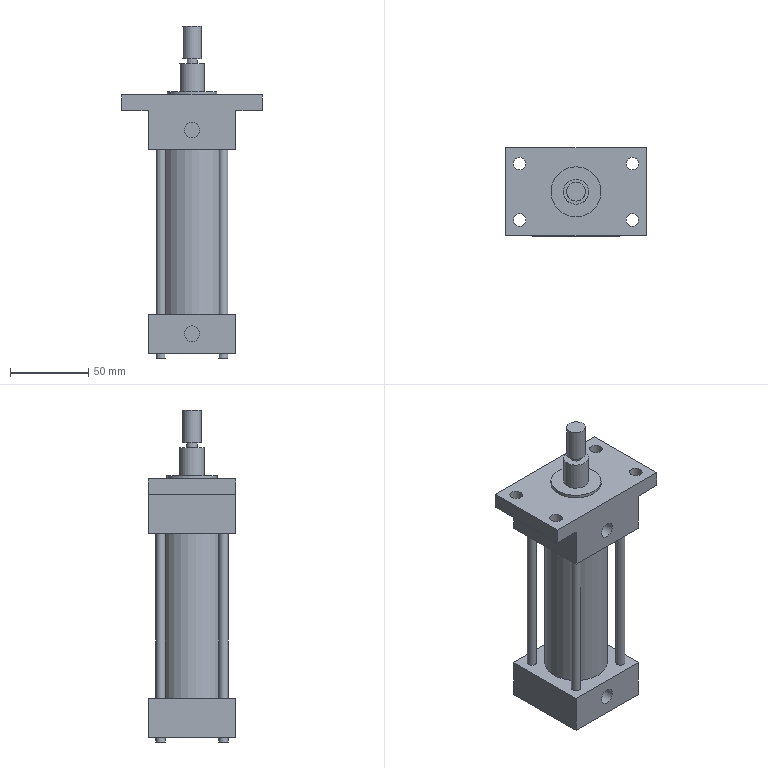Part | NX | features solid 2 | 1 solid | 48 faces | box 90 x 56 x 212 mm | volume 266006 mm3 | plane 28 | cylinder 20 | commonest cylinder face diameters 6 x8 8 x4 10 x2 7 x1 12 x1 16 x1
STEP:
#1=CARTESIAN_POINT('',(0.,-225.,-150.));
#2=VERTEX_POINT('',#1);
#3=CARTESIAN_POINT('',(0.,-245.,-150.));
#4=DIRECTION('',(0.,0.,1.));
#5=DIRECTION('',(0.,1.,0.));
#6=AXIS2_PLACEMENT_3D('',#3,#4,#5);
#7=CIRCLE('',#6,20.);
#8=EDGE_CURVE('',#2,#2,#7,.T.);
#9=ORIENTED_EDGE('',*,*,#8,.F.);
#10=EDGE_LOOP('',(#9));
#11=FACE_BOUND('',#10,.T.);
#12=CARTESIAN_POINT('',(0.,-225.,-255.));
#13=VERTEX_POINT('',#12);
#14=CARTESIAN_POINT('',(0.,-245.,-255.));
#15=DIRECTION('',(0.,0.,1.));
#16=DIRECTION('',(0.,1.,0.));
#17=AXIS2_PLACEMENT_3D('',#14,#15,#16);
#18=CIRCLE('',#17,20.);
#19=EDGE_CURVE('',#13,#13,#18,.F.);
#20=ORIENTED_EDGE('',*,*,#19,.F.);
#21=EDGE_LOOP('',(#20));
#22=FACE_BOUND('',#21,.T.);
#23=CARTESIAN_POINT('',(0.,-245.,-280.));
#24=DIRECTION('',(0.,0.,1.));
#25=DIRECTION('',(0.,-1.,0.));
#26=AXIS2_PLACEMENT_3D('',#23,#24,#25);
#27=CYLINDRICAL_SURFACE('',#26,20.);
#28=ADVANCED_FACE('',(#11,#22),#27,.T.);
#29=CARTESIAN_POINT('',(0.,-253.,-95.));
#30=VERTEX_POINT('',#29);
#31=CARTESIAN_POINT('',(0.,-245.,-95.));
#32=DIRECTION('',(0.,0.,-1.));
#33=DIRECTION('',(0.,-1.,0.));
#34=AXIS2_PLACEMENT_3D('',#31,#32,#33);
#35=CIRCLE('',#34,8.);
#36=EDGE_CURVE('',#30,#30,#35,.T.);
#37=ORIENTED_EDGE('',*,*,#36,.F.);
#38=EDGE_LOOP('',(#37));
#39=FACE_BOUND('',#38,.T.);
#40=CARTESIAN_POINT('',(0.,-248.5,-95.));
#41=VERTEX_POINT('',#40);
#42=CARTESIAN_POINT('',(0.,-245.,-95.));
#43=DIRECTION('',(0.,0.,-1.));
#44=DIRECTION('',(0.,-1.,0.));
#45=AXIS2_PLACEMENT_3D('',#42,#43,#44);
#46=CIRCLE('',#45,3.5);
#47=EDGE_CURVE('',#41,#41,#46,.T.);
#48=ORIENTED_EDGE('',*,*,#47,.T.);
#49=EDGE_LOOP('',(#48));
#50=FACE_BOUND('',#49,.T.);
#51=CARTESIAN_POINT('',(0.,-245.,-95.));
#52=DIRECTION('',(0.,0.,1.));
#53=DIRECTION('',(0.,-1.,0.));
#54=AXIS2_PLACEMENT_3D('',#51,#52,#53);
#55=PLANE('',#54);
#56=ADVANCED_FACE('',(#39,#50),#55,.T.);
#57=CARTESIAN_POINT('',(0.,-261.,-113.));
#58=VERTEX_POINT('',#57);
#59=CARTESIAN_POINT('',(0.,-245.,-113.));
#60=DIRECTION('',(0.,0.,-1.));
#61=DIRECTION('',(0.,-1.,0.));
#62=AXIS2_PLACEMENT_3D('',#59,#60,#61);
#63=CIRCLE('',#62,16.);
#64=EDGE_CURVE('',#58,#58,#63,.T.);
#65=ORIENTED_EDGE('',*,*,#64,.F.);
#66=EDGE_LOOP('',(#65));
#67=FACE_BOUND('',#66,.T.);
#68=CARTESIAN_POINT('',(0.,-253.,-113.));
#69=VERTEX_POINT('',#68);
#70=CARTESIAN_POINT('',(0.,-245.,-113.));
#71=DIRECTION('',(0.,0.,-1.));
#72=DIRECTION('',(0.,-1.,0.));
#73=AXIS2_PLACEMENT_3D('',#70,#71,#72);
#74=CIRCLE('',#73,8.);
#75=EDGE_CURVE('',#69,#69,#74,.F.);
#76=ORIENTED_EDGE('',*,*,#75,.F.);
#77=EDGE_LOOP('',(#76));
#78=FACE_BOUND('',#77,.T.);
#79=CARTESIAN_POINT('',(0.,-245.,-113.));
#80=DIRECTION('',(0.,0.,1.));
#81=DIRECTION('',(0.,-1.,0.));
#82=AXIS2_PLACEMENT_3D('',#79,#80,#81);
#83=PLANE('',#82);
#84=ADVANCED_FACE('',(#67,#78),#83,.T.);
#85=CARTESIAN_POINT('',(-36.,-231.,-115.));
#86=VERTEX_POINT('',#85);
#87=CARTESIAN_POINT('',(-36.,-227.,-115.));
#88=DIRECTION('',(0.,0.,-1.));
#89=DIRECTION('',(0.,-1.,0.));
#90=AXIS2_PLACEMENT_3D('',#87,#88,#89);
#91=CIRCLE('',#90,4.);
#92=EDGE_CURVE('',#86,#86,#91,.T.);
#93=ORIENTED_EDGE('',*,*,#92,.T.);
#94=EDGE_LOOP('',(#93));
#95=FACE_BOUND('',#94,.T.);
#96=CARTESIAN_POINT('',(36.,-267.,-115.));
#97=VERTEX_POINT('',#96);
#98=CARTESIAN_POINT('',(36.,-263.,-115.));
#99=DIRECTION('',(0.,0.,-1.));
#100=DIRECTION('',(0.,-1.,0.));
#101=AXIS2_PLACEMENT_3D('',#98,#99,#100);
#102=CIRCLE('',#101,4.);
#103=EDGE_CURVE('',#97,#97,#102,.T.);
#104=ORIENTED_EDGE('',*,*,#103,.T.);
#105=EDGE_LOOP('',(#104));
#106=FACE_BOUND('',#105,.T.);
#107=CARTESIAN_POINT('',(-45.,-217.,-115.));
#108=VERTEX_POINT('',#107);
#109=CARTESIAN_POINT('',(-45.,-273.,-115.));
#110=VERTEX_POINT('',#109);
#111=CARTESIAN_POINT('',(-45.,-217.,-115.));
#112=DIRECTION('',(0.,-1.,0.));
#113=VECTOR('',#112,1000.);
#114=LINE('',#111,#113);
#115=EDGE_CURVE('',#108,#110,#114,.T.);
#116=ORIENTED_EDGE('',*,*,#115,.T.);
#117=CARTESIAN_POINT('',(45.,-273.,-115.));
#118=VERTEX_POINT('',#117);
#119=CARTESIAN_POINT('',(45.,-273.,-115.));
#120=DIRECTION('',(-1.,0.,0.));
#121=VECTOR('',#120,1000.);
#122=LINE('',#119,#121);
#123=EDGE_CURVE('',#118,#110,#122,.T.);
#124=ORIENTED_EDGE('',*,*,#123,.F.);
#125=CARTESIAN_POINT('',(45.,-217.,-115.));
#126=VERTEX_POINT('',#125);
#127=CARTESIAN_POINT('',(45.,-217.,-115.));
#128=DIRECTION('',(0.,-1.,0.));
#129=VECTOR('',#128,1000.);
#130=LINE('',#127,#129);
#131=EDGE_CURVE('',#126,#118,#130,.T.);
#132=ORIENTED_EDGE('',*,*,#131,.F.);
#133=CARTESIAN_POINT('',(-28.,-217.,-115.));
#134=DIRECTION('',(-1.,0.,0.));
#135=VECTOR('',#134,1000.);
#136=LINE('',#133,#135);
#137=EDGE_CURVE('',#126,#108,#136,.T.);
#138=ORIENTED_EDGE('',*,*,#137,.T.);
#139=EDGE_LOOP('',(#116,#124,#132,#138));
#140=FACE_BOUND('',#139,.T.);
#141=CARTESIAN_POINT('',(36.,-231.,-115.));
#142=VERTEX_POINT('',#141);
#143=CARTESIAN_POINT('',(36.,-227.,-115.));
#144=DIRECTION('',(0.,0.,-1.));
#145=DIRECTION('',(0.,-1.,0.));
#146=AXIS2_PLACEMENT_3D('',#143,#144,#145);
#147=CIRCLE('',#146,4.);
#148=EDGE_CURVE('',#142,#142,#147,.T.);
#149=ORIENTED_EDGE('',*,*,#148,.T.);
#150=EDGE_LOOP('',(#149));
#151=FACE_BOUND('',#150,.T.);
#152=CARTESIAN_POINT('',(-36.,-267.,-115.));
#153=VERTEX_POINT('',#152);
#154=CARTESIAN_POINT('',(-36.,-263.,-115.));
#155=DIRECTION('',(0.,0.,-1.));
#156=DIRECTION('',(0.,-1.,0.));
#157=AXIS2_PLACEMENT_3D('',#154,#155,#156);
#158=CIRCLE('',#157,4.);
#159=EDGE_CURVE('',#153,#153,#158,.T.);
#160=ORIENTED_EDGE('',*,*,#159,.T.);
#161=EDGE_LOOP('',(#160));
#162=FACE_BOUND('',#161,.T.);
#163=CARTESIAN_POINT('',(0.,-229.,-115.));
#164=VERTEX_POINT('',#163);
#165=CARTESIAN_POINT('',(0.,-245.,-115.));
#166=DIRECTION('',(0.,0.,1.));
#167=DIRECTION('',(0.,1.,0.));
#168=AXIS2_PLACEMENT_3D('',#165,#166,#167);
#169=CIRCLE('',#168,16.);
#170=EDGE_CURVE('',#164,#164,#169,.F.);
#171=ORIENTED_EDGE('',*,*,#170,.T.);
#172=EDGE_LOOP('',(#171));
#173=FACE_BOUND('',#172,.T.);
#174=CARTESIAN_POINT('',(-45.,-273.,-115.));
#175=DIRECTION('',(0.,0.,-1.));
#176=DIRECTION('',(0.,1.,0.));
#177=AXIS2_PLACEMENT_3D('',#174,#175,#176);
#178=PLANE('',#177);
#179=ADVANCED_FACE('',(#95,#106,#140,#151,#162,#173),#178,.F.);
#180=CARTESIAN_POINT('',(28.,-273.,-125.));
#181=VERTEX_POINT('',#180);
#182=CARTESIAN_POINT('',(28.,-217.,-125.));
#183=VERTEX_POINT('',#182);
#184=CARTESIAN_POINT('',(28.,-273.,-125.));
#185=DIRECTION('',(0.,1.,0.));
#186=VECTOR('',#185,1000.);
#187=LINE('',#184,#186);
#188=EDGE_CURVE('',#181,#183,#187,.T.);
#189=ORIENTED_EDGE('',*,*,#188,.T.);
#190=CARTESIAN_POINT('',(45.,-217.,-125.));
#191=VERTEX_POINT('',#190);
#192=CARTESIAN_POINT('',(-28.,-217.,-125.));
#193=DIRECTION('',(-1.,0.,0.));
#194=VECTOR('',#193,1000.);
#195=LINE('',#192,#194);
#196=EDGE_CURVE('',#191,#183,#195,.T.);
#197=ORIENTED_EDGE('',*,*,#196,.F.);
#198=CARTESIAN_POINT('',(45.,-273.,-125.));
#199=VERTEX_POINT('',#198);
#200=CARTESIAN_POINT('',(45.,-217.,-125.));
#201=DIRECTION('',(0.,-1.,0.));
#202=VECTOR('',#201,1000.);
#203=LINE('',#200,#202);
#204=EDGE_CURVE('',#191,#199,#203,.T.);
#205=ORIENTED_EDGE('',*,*,#204,.T.);
#206=CARTESIAN_POINT('',(45.,-273.,-125.));
#207=DIRECTION('',(-1.,0.,0.));
#208=VECTOR('',#207,1000.);
#209=LINE('',#206,#208);
#210=EDGE_CURVE('',#199,#181,#209,.T.);
#211=ORIENTED_EDGE('',*,*,#210,.T.);
#212=EDGE_LOOP('',(#189,#197,#205,#211));
#213=FACE_BOUND('',#212,.T.);
#214=CARTESIAN_POINT('',(36.,-267.,-125.));
#215=VERTEX_POINT('',#214);
#216=CARTESIAN_POINT('',(36.,-263.,-125.));
#217=DIRECTION('',(0.,0.,-1.));
#218=DIRECTION('',(0.,-1.,0.));
#219=AXIS2_PLACEMENT_3D('',#216,#217,#218);
#220=CIRCLE('',#219,4.);
#221=EDGE_CURVE('',#215,#215,#220,.T.);
#222=ORIENTED_EDGE('',*,*,#221,.F.);
#223=EDGE_LOOP('',(#222));
#224=FACE_BOUND('',#223,.T.);
#225=CARTESIAN_POINT('',(36.,-231.,-125.));
#226=VERTEX_POINT('',#225);
#227=CARTESIAN_POINT('',(36.,-227.,-125.));
#228=DIRECTION('',(0.,0.,-1.));
#229=DIRECTION('',(0.,-1.,0.));
#230=AXIS2_PLACEMENT_3D('',#227,#228,#229);
#231=CIRCLE('',#230,4.);
#232=EDGE_CURVE('',#226,#226,#231,.T.);
#233=ORIENTED_EDGE('',*,*,#232,.F.);
#234=EDGE_LOOP('',(#233));
#235=FACE_BOUND('',#234,.T.);
#236=CARTESIAN_POINT('',(-45.,-273.,-125.));
#237=DIRECTION('',(0.,0.,-1.));
#238=DIRECTION('',(0.,1.,0.));
#239=AXIS2_PLACEMENT_3D('',#236,#237,#238);
#240=PLANE('',#239);
#241=ADVANCED_FACE('',(#213,#224,#235),#240,.T.);
#242=ORIENTED_EDGE('',*,*,#115,.F.);
#243=CARTESIAN_POINT('',(-45.,-217.,-125.));
#244=VERTEX_POINT('',#243);
#245=CARTESIAN_POINT('',(-45.,-217.,-125.));
#246=DIRECTION('',(0.,0.,1.));
#247=VECTOR('',#246,1000.);
#248=LINE('',#245,#247);
#249=EDGE_CURVE('',#244,#108,#248,.T.);
#250=ORIENTED_EDGE('',*,*,#249,.F.);
#251=CARTESIAN_POINT('',(-45.,-273.,-125.));
#252=VERTEX_POINT('',#251);
#253=CARTESIAN_POINT('',(-45.,-217.,-125.));
#254=DIRECTION('',(0.,-1.,0.));
#255=VECTOR('',#254,1000.);
#256=LINE('',#253,#255);
#257=EDGE_CURVE('',#244,#252,#256,.T.);
#258=ORIENTED_EDGE('',*,*,#257,.T.);
#259=CARTESIAN_POINT('',(-45.,-273.,-125.));
#260=DIRECTION('',(0.,0.,1.));
#261=VECTOR('',#260,1000.);
#262=LINE('',#259,#261);
#263=EDGE_CURVE('',#252,#110,#262,.T.);
#264=ORIENTED_EDGE('',*,*,#263,.T.);
#265=EDGE_LOOP('',(#242,#250,#258,#264));
#266=FACE_BOUND('',#265,.T.);
#267=CARTESIAN_POINT('',(-45.,-217.,-125.));
#268=DIRECTION('',(1.,0.,0.));
#269=DIRECTION('',(0.,0.,-1.));
#270=AXIS2_PLACEMENT_3D('',#267,#268,#269);
#271=PLANE('',#270);
#272=ADVANCED_FACE('',(#266),#271,.F.);
#273=CARTESIAN_POINT('',(5.,-273.,-137.5));
#274=VERTEX_POINT('',#273);
#275=CARTESIAN_POINT('',(0.,-273.,-137.5));
#276=DIRECTION('',(0.,-1.,0.));
#277=DIRECTION('',(1.,0.,0.));
#278=AXIS2_PLACEMENT_3D('',#275,#276,#277);
#279=CIRCLE('',#278,5.);
#280=EDGE_CURVE('',#274,#274,#279,.T.);
#281=ORIENTED_EDGE('',*,*,#280,.F.);
#282=EDGE_LOOP('',(#281));
#283=FACE_BOUND('',#282,.T.);
#284=ORIENTED_EDGE('',*,*,#123,.T.);
#285=ORIENTED_EDGE('',*,*,#263,.F.);
#286=CARTESIAN_POINT('',(-28.,-273.,-125.));
#287=VERTEX_POINT('',#286);
#288=CARTESIAN_POINT('',(45.,-273.,-125.));
#289=DIRECTION('',(-1.,0.,0.));
#290=VECTOR('',#289,1000.);
#291=LINE('',#288,#290);
#292=EDGE_CURVE('',#287,#252,#291,.T.);
#293=ORIENTED_EDGE('',*,*,#292,.F.);
#294=CARTESIAN_POINT('',(-28.,-273.,-150.));
#295=VERTEX_POINT('',#294);
#296=CARTESIAN_POINT('',(-28.,-273.,-150.));
#297=DIRECTION('',(0.,0.,1.));
#298=VECTOR('',#297,1000.);
#299=LINE('',#296,#298);
#300=EDGE_CURVE('',#295,#287,#299,.T.);
#301=ORIENTED_EDGE('',*,*,#300,.F.);
#302=CARTESIAN_POINT('',(28.,-273.,-150.));
#303=VERTEX_POINT('',#302);
#304=CARTESIAN_POINT('',(-28.,-273.,-150.));
#305=DIRECTION('',(1.,0.,0.));
#306=VECTOR('',#305,1000.);
#307=LINE('',#304,#306);
#308=EDGE_CURVE('',#295,#303,#307,.T.);
#309=ORIENTED_EDGE('',*,*,#308,.T.);
#310=CARTESIAN_POINT('',(28.,-273.,-150.));
#311=DIRECTION('',(0.,0.,1.));
#312=VECTOR('',#311,1000.);
#313=LINE('',#310,#312);
#314=EDGE_CURVE('',#303,#181,#313,.T.);
#315=ORIENTED_EDGE('',*,*,#314,.T.);
#316=ORIENTED_EDGE('',*,*,#210,.F.);
#317=CARTESIAN_POINT('',(45.,-273.,-125.));
#318=DIRECTION('',(0.,0.,1.));
#319=VECTOR('',#318,1000.);
#320=LINE('',#317,#319);
#321=EDGE_CURVE('',#199,#118,#320,.T.);
#322=ORIENTED_EDGE('',*,*,#321,.T.);
#323=EDGE_LOOP('',(#284,#285,#293,#301,#309,#315,#316,#322));
#324=FACE_BOUND('',#323,.T.);
#325=CARTESIAN_POINT('',(45.,-273.,-125.));
#326=DIRECTION('',(0.,-1.,0.));
#327=DIRECTION('',(-1.,0.,0.));
#328=AXIS2_PLACEMENT_3D('',#325,#326,#327);
#329=PLANE('',#328);
#330=ADVANCED_FACE('',(#283,#324),#329,.T.);
#331=ORIENTED_EDGE('',*,*,#131,.T.);
#332=ORIENTED_EDGE('',*,*,#321,.F.);
#333=ORIENTED_EDGE('',*,*,#204,.F.);
#334=CARTESIAN_POINT('',(45.,-217.,-125.));
#335=DIRECTION('',(0.,0.,1.));
#336=VECTOR('',#335,1000.);
#337=LINE('',#334,#336);
#338=EDGE_CURVE('',#191,#126,#337,.T.);
#339=ORIENTED_EDGE('',*,*,#338,.T.);
#340=EDGE_LOOP('',(#331,#332,#333,#339));
#341=FACE_BOUND('',#340,.T.);
#342=CARTESIAN_POINT('',(45.,-217.,-125.));
#343=DIRECTION('',(1.,0.,0.));
#344=DIRECTION('',(0.,0.,-1.));
#345=AXIS2_PLACEMENT_3D('',#342,#343,#344);
#346=PLANE('',#345);
#347=ADVANCED_FACE('',(#341),#346,.T.);
#348=ORIENTED_EDGE('',*,*,#221,.T.);
#349=EDGE_LOOP('',(#348));
#350=FACE_BOUND('',#349,.T.);
#351=ORIENTED_EDGE('',*,*,#103,.F.);
#352=EDGE_LOOP('',(#351));
#353=FACE_BOUND('',#352,.T.);
#354=CARTESIAN_POINT('',(36.,-263.,-125.));
#355=DIRECTION('',(0.,0.,1.));
#356=DIRECTION('',(0.,-1.,0.));
#357=AXIS2_PLACEMENT_3D('',#354,#355,#356);
#358=CYLINDRICAL_SURFACE('',#357,4.);
#359=ADVANCED_FACE('',(#350,#353),#358,.F.);
#360=ORIENTED_EDGE('',*,*,#137,.F.);
#361=ORIENTED_EDGE('',*,*,#338,.F.);
#362=ORIENTED_EDGE('',*,*,#196,.T.);
#363=CARTESIAN_POINT('',(28.,-217.,-150.));
#364=VERTEX_POINT('',#363);
#365=CARTESIAN_POINT('',(28.,-217.,-150.));
#366=DIRECTION('',(0.,0.,1.));
#367=VECTOR('',#366,1000.);
#368=LINE('',#365,#367);
#369=EDGE_CURVE('',#364,#183,#368,.T.);
#370=ORIENTED_EDGE('',*,*,#369,.F.);
#371=CARTESIAN_POINT('',(-28.,-217.,-150.));
#372=VERTEX_POINT('',#371);
#373=CARTESIAN_POINT('',(28.,-217.,-150.));
#374=DIRECTION('',(-1.,0.,0.));
#375=VECTOR('',#374,1000.);
#376=LINE('',#373,#375);
#377=EDGE_CURVE('',#364,#372,#376,.T.);
#378=ORIENTED_EDGE('',*,*,#377,.T.);
#379=CARTESIAN_POINT('',(-28.,-217.,-125.));
#380=VERTEX_POINT('',#379);
#381=CARTESIAN_POINT('',(-28.,-217.,-150.));
#382=DIRECTION('',(0.,0.,1.));
#383=VECTOR('',#382,1000.);
#384=LINE('',#381,#383);
#385=EDGE_CURVE('',#372,#380,#384,.T.);
#386=ORIENTED_EDGE('',*,*,#385,.T.);
#387=CARTESIAN_POINT('',(-28.,-217.,-125.));
#388=DIRECTION('',(-1.,0.,0.));
#389=VECTOR('',#388,1000.);
#390=LINE('',#387,#389);
#391=EDGE_CURVE('',#380,#244,#390,.T.);
#392=ORIENTED_EDGE('',*,*,#391,.T.);
#393=ORIENTED_EDGE('',*,*,#249,.T.);
#394=EDGE_LOOP('',(#360,#361,#362,#370,#378,#386,#392,#393));
#395=FACE_BOUND('',#394,.T.);
#396=CARTESIAN_POINT('',(-28.,-217.,-125.));
#397=DIRECTION('',(0.,-1.,0.));
#398=DIRECTION('',(0.,0.,-1.));
#399=AXIS2_PLACEMENT_3D('',#396,#397,#398);
#400=PLANE('',#399);
#401=ADVANCED_FACE('',(#395),#400,.F.);
#402=ORIENTED_EDGE('',*,*,#232,.T.);
#403=EDGE_LOOP('',(#402));
#404=FACE_BOUND('',#403,.T.);
#405=ORIENTED_EDGE('',*,*,#148,.F.);
#406=EDGE_LOOP('',(#405));
#407=FACE_BOUND('',#406,.T.);
#408=CARTESIAN_POINT('',(36.,-227.,-125.));
#409=DIRECTION('',(0.,0.,1.));
#410=DIRECTION('',(0.,-1.,0.));
#411=AXIS2_PLACEMENT_3D('',#408,#409,#410);
#412=CYLINDRICAL_SURFACE('',#411,4.);
#413=ADVANCED_FACE('',(#404,#407),#412,.F.);
#414=CARTESIAN_POINT('',(-36.,-267.,-125.));
#415=VERTEX_POINT('',#414);
#416=CARTESIAN_POINT('',(-36.,-263.,-125.));
#417=DIRECTION('',(0.,0.,-1.));
#418=DIRECTION('',(0.,-1.,0.));
#419=AXIS2_PLACEMENT_3D('',#416,#417,#418);
#420=CIRCLE('',#419,4.);
#421=EDGE_CURVE('',#415,#415,#420,.T.);
#422=ORIENTED_EDGE('',*,*,#421,.T.);
#423=EDGE_LOOP('',(#422));
#424=FACE_BOUND('',#423,.T.);
#425=ORIENTED_EDGE('',*,*,#159,.F.);
#426=EDGE_LOOP('',(#425));
#427=FACE_BOUND('',#426,.T.);
#428=CARTESIAN_POINT('',(-36.,-263.,-125.));
#429=DIRECTION('',(0.,0.,1.));
#430=DIRECTION('',(0.,-1.,0.));
#431=AXIS2_PLACEMENT_3D('',#428,#429,#430);
#432=CYLINDRICAL_SURFACE('',#431,4.);
#433=ADVANCED_FACE('',(#424,#427),#432,.F.);
#434=CARTESIAN_POINT('',(-36.,-231.,-125.));
#435=VERTEX_POINT('',#434);
#436=CARTESIAN_POINT('',(-36.,-227.,-125.));
#437=DIRECTION('',(0.,0.,-1.));
#438=DIRECTION('',(0.,-1.,0.));
#439=AXIS2_PLACEMENT_3D('',#436,#437,#438);
#440=CIRCLE('',#439,4.);
#441=EDGE_CURVE('',#435,#435,#440,.T.);
#442=ORIENTED_EDGE('',*,*,#441,.T.);
#443=EDGE_LOOP('',(#442));
#444=FACE_BOUND('',#443,.T.);
#445=ORIENTED_EDGE('',*,*,#92,.F.);
#446=EDGE_LOOP('',(#445));
#447=FACE_BOUND('',#446,.T.);
#448=CARTESIAN_POINT('',(-36.,-227.,-125.));
#449=DIRECTION('',(0.,0.,1.));
#450=DIRECTION('',(0.,-1.,0.));
#451=AXIS2_PLACEMENT_3D('',#448,#449,#450);
#452=CYLINDRICAL_SURFACE('',#451,4.);
#453=ADVANCED_FACE('',(#444,#447),#452,.F.);
#454=CARTESIAN_POINT('',(-28.,-217.,-125.));
#455=DIRECTION('',(0.,-1.,0.));
#456=VECTOR('',#455,1000.);
#457=LINE('',#454,#456);
#458=EDGE_CURVE('',#380,#287,#457,.T.);
#459=ORIENTED_EDGE('',*,*,#458,.T.);
#460=ORIENTED_EDGE('',*,*,#292,.T.);
#461=ORIENTED_EDGE('',*,*,#257,.F.);
#462=ORIENTED_EDGE('',*,*,#391,.F.);
#463=EDGE_LOOP('',(#459,#460,#461,#462));
#464=FACE_BOUND('',#463,.T.);
#465=ORIENTED_EDGE('',*,*,#421,.F.);
#466=EDGE_LOOP('',(#465));
#467=FACE_BOUND('',#466,.T.);
#468=ORIENTED_EDGE('',*,*,#441,.F.);
#469=EDGE_LOOP('',(#468));
#470=FACE_BOUND('',#469,.T.);
#471=CARTESIAN_POINT('',(-45.,-273.,-125.));
#472=DIRECTION('',(0.,0.,-1.));
#473=DIRECTION('',(0.,1.,0.));
#474=AXIS2_PLACEMENT_3D('',#471,#472,#473);
#475=PLANE('',#474);
#476=ADVANCED_FACE('',(#464,#467,#470),#475,.T.);
#477=ORIENTED_EDGE('',*,*,#458,.F.);
#478=ORIENTED_EDGE('',*,*,#385,.F.);
#479=CARTESIAN_POINT('',(-28.,-217.,-150.));
#480=DIRECTION('',(0.,-1.,0.));
#481=VECTOR('',#480,1000.);
#482=LINE('',#479,#481);
#483=EDGE_CURVE('',#372,#295,#482,.T.);
#484=ORIENTED_EDGE('',*,*,#483,.T.);
#485=ORIENTED_EDGE('',*,*,#300,.T.);
#486=EDGE_LOOP('',(#477,#478,#484,#485));
#487=FACE_BOUND('',#486,.T.);
#488=CARTESIAN_POINT('',(-28.,-217.,-150.));
#489=DIRECTION('',(1.,0.,0.));
#490=DIRECTION('',(0.,0.,-1.));
#491=AXIS2_PLACEMENT_3D('',#488,#489,#490);
#492=PLANE('',#491);
#493=ADVANCED_FACE('',(#487),#492,.F.);
#494=ORIENTED_EDGE('',*,*,#188,.F.);
#495=ORIENTED_EDGE('',*,*,#314,.F.);
#496=CARTESIAN_POINT('',(28.,-273.,-150.));
#497=DIRECTION('',(0.,1.,0.));
#498=VECTOR('',#497,1000.);
#499=LINE('',#496,#498);
#500=EDGE_CURVE('',#303,#364,#499,.T.);
#501=ORIENTED_EDGE('',*,*,#500,.T.);
#502=ORIENTED_EDGE('',*,*,#369,.T.);
#503=EDGE_LOOP('',(#494,#495,#501,#502));
#504=FACE_BOUND('',#503,.T.);
#505=CARTESIAN_POINT('',(28.,-273.,-150.));
#506=DIRECTION('',(-1.,0.,0.));
#507=DIRECTION('',(0.,0.,1.));
#508=AXIS2_PLACEMENT_3D('',#505,#506,#507);
#509=PLANE('',#508);
#510=ADVANCED_FACE('',(#504),#509,.F.);
#511=CARTESIAN_POINT('',(-20.,-262.,-150.));
#512=VERTEX_POINT('',#511);
#513=CARTESIAN_POINT('',(-20.,-265.,-150.));
#514=DIRECTION('',(0.,0.,1.));
#515=DIRECTION('',(0.,1.,0.));
#516=AXIS2_PLACEMENT_3D('',#513,#514,#515);
#517=CIRCLE('',#516,3.);
#518=EDGE_CURVE('',#512,#512,#517,.T.);
#519=ORIENTED_EDGE('',*,*,#518,.T.);
#520=EDGE_LOOP('',(#519));
#521=FACE_BOUND('',#520,.T.);
#522=CARTESIAN_POINT('',(-20.,-222.,-150.));
#523=VERTEX_POINT('',#522);
#524=CARTESIAN_POINT('',(-20.,-225.,-150.));
#525=DIRECTION('',(0.,0.,1.));
#526=DIRECTION('',(0.,1.,0.));
#527=AXIS2_PLACEMENT_3D('',#524,#525,#526);
#528=CIRCLE('',#527,3.);
#529=EDGE_CURVE('',#523,#523,#528,.T.);
#530=ORIENTED_EDGE('',*,*,#529,.T.);
#531=EDGE_LOOP('',(#530));
#532=FACE_BOUND('',#531,.T.);
#533=CARTESIAN_POINT('',(20.,-222.,-150.));
#534=VERTEX_POINT('',#533);
#535=CARTESIAN_POINT('',(20.,-225.,-150.));
#536=DIRECTION('',(0.,0.,1.));
#537=DIRECTION('',(0.,1.,0.));
#538=AXIS2_PLACEMENT_3D('',#535,#536,#537);
#539=CIRCLE('',#538,3.);
#540=EDGE_CURVE('',#534,#534,#539,.T.);
#541=ORIENTED_EDGE('',*,*,#540,.T.);
#542=EDGE_LOOP('',(#541));
#543=FACE_BOUND('',#542,.T.);
#544=CARTESIAN_POINT('',(20.,-262.,-150.));
#545=VERTEX_POINT('',#544);
#546=CARTESIAN_POINT('',(20.,-265.,-150.));
#547=DIRECTION('',(0.,0.,1.));
#548=DIRECTION('',(0.,1.,0.));
#549=AXIS2_PLACEMENT_3D('',#546,#547,#548);
#550=CIRCLE('',#549,3.);
#551=EDGE_CURVE('',#545,#545,#550,.T.);
#552=ORIENTED_EDGE('',*,*,#551,.T.);
#553=EDGE_LOOP('',(#552));
#554=FACE_BOUND('',#553,.T.);
#555=ORIENTED_EDGE('',*,*,#8,.T.);
#556=EDGE_LOOP('',(#555));
#557=FACE_BOUND('',#556,.T.);
#558=ORIENTED_EDGE('',*,*,#377,.F.);
#559=ORIENTED_EDGE('',*,*,#500,.F.);
#560=ORIENTED_EDGE('',*,*,#308,.F.);
#561=ORIENTED_EDGE('',*,*,#483,.F.);
#562=EDGE_LOOP('',(#558,#559,#560,#561));
#563=FACE_BOUND('',#562,.T.);
#564=CARTESIAN_POINT('',(-28.,-217.,-150.));
#565=DIRECTION('',(0.,0.,-1.));
#566=DIRECTION('',(0.,1.,0.));
#567=AXIS2_PLACEMENT_3D('',#564,#565,#566);
#568=PLANE('',#567);
#569=ADVANCED_FACE('',(#521,#532,#543,#554,#557,#563),#568,.T.);
#570=ORIENTED_EDGE('',*,*,#64,.T.);
#571=EDGE_LOOP('',(#570));
#572=FACE_BOUND('',#571,.T.);
#573=ORIENTED_EDGE('',*,*,#170,.F.);
#574=EDGE_LOOP('',(#573));
#575=FACE_BOUND('',#574,.T.);
#576=CARTESIAN_POINT('',(0.,-245.,-113.));
#577=DIRECTION('',(0.,0.,-1.));
#578=DIRECTION('',(0.,1.,0.));
#579=AXIS2_PLACEMENT_3D('',#576,#577,#578);
#580=CYLINDRICAL_SURFACE('',#579,16.);
#581=ADVANCED_FACE('',(#572,#575),#580,.T.);
#582=ORIENTED_EDGE('',*,*,#75,.T.);
#583=EDGE_LOOP('',(#582));
#584=FACE_BOUND('',#583,.T.);
#585=ORIENTED_EDGE('',*,*,#36,.T.);
#586=EDGE_LOOP('',(#585));
#587=FACE_BOUND('',#586,.T.);
#588=CARTESIAN_POINT('',(0.,-245.,-95.));
#589=DIRECTION('',(0.,0.,-1.));
#590=DIRECTION('',(0.,1.,0.));
#591=AXIS2_PLACEMENT_3D('',#588,#589,#590);
#592=CYLINDRICAL_SURFACE('',#591,8.);
#593=ADVANCED_FACE('',(#584,#587),#592,.T.);
#594=CARTESIAN_POINT('',(28.,-217.,-255.));
#595=VERTEX_POINT('',#594);
#596=CARTESIAN_POINT('',(-28.,-217.,-255.));
#597=VERTEX_POINT('',#596);
#598=CARTESIAN_POINT('',(28.,-217.,-255.));
#599=DIRECTION('',(-1.,0.,0.));
#600=VECTOR('',#599,1000.);
#601=LINE('',#598,#600);
#602=EDGE_CURVE('',#595,#597,#601,.T.);
#603=ORIENTED_EDGE('',*,*,#602,.F.);
#604=CARTESIAN_POINT('',(28.,-217.,-280.));
#605=VERTEX_POINT('',#604);
#606=CARTESIAN_POINT('',(28.,-217.,-280.));
#607=DIRECTION('',(0.,0.,1.));
#608=VECTOR('',#607,1000.);
#609=LINE('',#606,#608);
#610=EDGE_CURVE('',#605,#595,#609,.T.);
#611=ORIENTED_EDGE('',*,*,#610,.F.);
#612=CARTESIAN_POINT('',(-28.,-217.,-280.));
#613=VERTEX_POINT('',#612);
#614=CARTESIAN_POINT('',(28.,-217.,-280.));
#615=DIRECTION('',(-1.,0.,0.));
#616=VECTOR('',#615,1000.);
#617=LINE('',#614,#616);
#618=EDGE_CURVE('',#605,#613,#617,.T.);
#619=ORIENTED_EDGE('',*,*,#618,.T.);
#620=CARTESIAN_POINT('',(-28.,-217.,-280.));
#621=DIRECTION('',(0.,0.,1.));
#622=VECTOR('',#621,1000.);
#623=LINE('',#620,#622);
#624=EDGE_CURVE('',#613,#597,#623,.T.);
#625=ORIENTED_EDGE('',*,*,#624,.T.);
#626=EDGE_LOOP('',(#603,#611,#619,#625));
#627=FACE_BOUND('',#626,.T.);
#628=CARTESIAN_POINT('',(28.,-217.,-280.));
#629=DIRECTION('',(0.,-1.,0.));
#630=DIRECTION('',(0.,0.,-1.));
#631=AXIS2_PLACEMENT_3D('',#628,#629,#630);
#632=PLANE('',#631);
#633=ADVANCED_FACE('',(#627),#632,.F.);
#634=CARTESIAN_POINT('',(-28.,-273.,-255.));
#635=VERTEX_POINT('',#634);
#636=CARTESIAN_POINT('',(-28.,-217.,-255.));
#637=DIRECTION('',(0.,-1.,0.));
#638=VECTOR('',#637,1000.);
#639=LINE('',#636,#638);
#640=EDGE_CURVE('',#597,#635,#639,.T.);
#641=ORIENTED_EDGE('',*,*,#640,.F.);
#642=ORIENTED_EDGE('',*,*,#624,.F.);
#643=CARTESIAN_POINT('',(-28.,-273.,-280.));
#644=VERTEX_POINT('',#643);
#645=CARTESIAN_POINT('',(-28.,-217.,-280.));
#646=DIRECTION('',(0.,-1.,0.));
#647=VECTOR('',#646,1000.);
#648=LINE('',#645,#647);
#649=EDGE_CURVE('',#613,#644,#648,.T.);
#650=ORIENTED_EDGE('',*,*,#649,.T.);
#651=CARTESIAN_POINT('',(-28.,-273.,-280.));
#652=DIRECTION('',(0.,0.,1.));
#653=VECTOR('',#652,1000.);
#654=LINE('',#651,#653);
#655=EDGE_CURVE('',#644,#635,#654,.T.);
#656=ORIENTED_EDGE('',*,*,#655,.T.);
#657=EDGE_LOOP('',(#641,#642,#650,#656));
#658=FACE_BOUND('',#657,.T.);
#659=CARTESIAN_POINT('',(-28.,-217.,-280.));
#660=DIRECTION('',(1.,0.,0.));
#661=DIRECTION('',(0.,0.,-1.));
#662=AXIS2_PLACEMENT_3D('',#659,#660,#661);
#663=PLANE('',#662);
#664=ADVANCED_FACE('',(#658),#663,.F.);
#665=CARTESIAN_POINT('',(5.,-273.,-267.5));
#666=VERTEX_POINT('',#665);
#667=CARTESIAN_POINT('',(0.,-273.,-267.5));
#668=DIRECTION('',(0.,-1.,0.));
#669=DIRECTION('',(1.,0.,0.));
#670=AXIS2_PLACEMENT_3D('',#667,#668,#669);
#671=CIRCLE('',#670,5.);
#672=EDGE_CURVE('',#666,#666,#671,.T.);
#673=ORIENTED_EDGE('',*,*,#672,.F.);
#674=EDGE_LOOP('',(#673));
#675=FACE_BOUND('',#674,.T.);
#676=CARTESIAN_POINT('',(28.,-273.,-255.));
#677=VERTEX_POINT('',#676);
#678=CARTESIAN_POINT('',(-28.,-273.,-255.));
#679=DIRECTION('',(1.,0.,0.));
#680=VECTOR('',#679,1000.);
#681=LINE('',#678,#680);
#682=EDGE_CURVE('',#635,#677,#681,.T.);
#683=ORIENTED_EDGE('',*,*,#682,.F.);
#684=ORIENTED_EDGE('',*,*,#655,.F.);
#685=CARTESIAN_POINT('',(28.,-273.,-280.));
#686=VERTEX_POINT('',#685);
#687=CARTESIAN_POINT('',(-28.,-273.,-280.));
#688=DIRECTION('',(1.,0.,0.));
#689=VECTOR('',#688,1000.);
#690=LINE('',#687,#689);
#691=EDGE_CURVE('',#644,#686,#690,.T.);
#692=ORIENTED_EDGE('',*,*,#691,.T.);
#693=CARTESIAN_POINT('',(28.,-273.,-280.));
#694=DIRECTION('',(0.,0.,1.));
#695=VECTOR('',#694,1000.);
#696=LINE('',#693,#695);
#697=EDGE_CURVE('',#686,#677,#696,.T.);
#698=ORIENTED_EDGE('',*,*,#697,.T.);
#699=EDGE_LOOP('',(#683,#684,#692,#698));
#700=FACE_BOUND('',#699,.T.);
#701=CARTESIAN_POINT('',(-28.,-273.,-280.));
#702=DIRECTION('',(0.,1.,0.));
#703=DIRECTION('',(1.,0.,0.));
#704=AXIS2_PLACEMENT_3D('',#701,#702,#703);
#705=PLANE('',#704);
#706=ADVANCED_FACE('',(#675,#700),#705,.F.);
#707=CARTESIAN_POINT('',(28.,-273.,-255.));
#708=DIRECTION('',(0.,1.,0.));
#709=VECTOR('',#708,1000.);
#710=LINE('',#707,#709);
#711=EDGE_CURVE('',#677,#595,#710,.T.);
#712=ORIENTED_EDGE('',*,*,#711,.F.);
#713=ORIENTED_EDGE('',*,*,#697,.F.);
#714=CARTESIAN_POINT('',(28.,-273.,-280.));
#715=DIRECTION('',(0.,1.,0.));
#716=VECTOR('',#715,1000.);
#717=LINE('',#714,#716);
#718=EDGE_CURVE('',#686,#605,#717,.T.);
#719=ORIENTED_EDGE('',*,*,#718,.T.);
#720=ORIENTED_EDGE('',*,*,#610,.T.);
#721=EDGE_LOOP('',(#712,#713,#719,#720));
#722=FACE_BOUND('',#721,.T.);
#723=CARTESIAN_POINT('',(28.,-273.,-280.));
#724=DIRECTION('',(-1.,0.,0.));
#725=DIRECTION('',(0.,0.,1.));
#726=AXIS2_PLACEMENT_3D('',#723,#724,#725);
#727=PLANE('',#726);
#728=ADVANCED_FACE('',(#722),#727,.F.);
#729=CARTESIAN_POINT('',(-20.,-262.,-255.));
#730=VERTEX_POINT('',#729);
#731=CARTESIAN_POINT('',(-20.,-265.,-255.));
#732=DIRECTION('',(0.,0.,1.));
#733=DIRECTION('',(0.,1.,0.));
#734=AXIS2_PLACEMENT_3D('',#731,#732,#733);
#735=CIRCLE('',#734,3.);
#736=EDGE_CURVE('',#730,#730,#735,.T.);
#737=ORIENTED_EDGE('',*,*,#736,.F.);
#738=EDGE_LOOP('',(#737));
#739=FACE_BOUND('',#738,.T.);
#740=CARTESIAN_POINT('',(-20.,-222.,-255.));
#741=VERTEX_POINT('',#740);
#742=CARTESIAN_POINT('',(-20.,-225.,-255.));
#743=DIRECTION('',(0.,0.,1.));
#744=DIRECTION('',(0.,1.,0.));
#745=AXIS2_PLACEMENT_3D('',#742,#743,#744);
#746=CIRCLE('',#745,3.);
#747=EDGE_CURVE('',#741,#741,#746,.T.);
#748=ORIENTED_EDGE('',*,*,#747,.F.);
#749=EDGE_LOOP('',(#748));
#750=FACE_BOUND('',#749,.T.);
#751=CARTESIAN_POINT('',(20.,-222.,-255.));
#752=VERTEX_POINT('',#751);
#753=CARTESIAN_POINT('',(20.,-225.,-255.));
#754=DIRECTION('',(0.,0.,1.));
#755=DIRECTION('',(0.,1.,0.));
#756=AXIS2_PLACEMENT_3D('',#753,#754,#755);
#757=CIRCLE('',#756,3.);
#758=EDGE_CURVE('',#752,#752,#757,.T.);
#759=ORIENTED_EDGE('',*,*,#758,.F.);
#760=EDGE_LOOP('',(#759));
#761=FACE_BOUND('',#760,.T.);
#762=CARTESIAN_POINT('',(20.,-262.,-255.));
#763=VERTEX_POINT('',#762);
#764=CARTESIAN_POINT('',(20.,-265.,-255.));
#765=DIRECTION('',(0.,0.,1.));
#766=DIRECTION('',(0.,1.,0.));
#767=AXIS2_PLACEMENT_3D('',#764,#765,#766);
#768=CIRCLE('',#767,3.);
#769=EDGE_CURVE('',#763,#763,#768,.T.);
#770=ORIENTED_EDGE('',*,*,#769,.F.);
#771=EDGE_LOOP('',(#770));
#772=FACE_BOUND('',#771,.T.);
#773=ORIENTED_EDGE('',*,*,#19,.T.);
#774=EDGE_LOOP('',(#773));
#775=FACE_BOUND('',#774,.T.);
#776=ORIENTED_EDGE('',*,*,#602,.T.);
#777=ORIENTED_EDGE('',*,*,#640,.T.);
#778=ORIENTED_EDGE('',*,*,#682,.T.);
#779=ORIENTED_EDGE('',*,*,#711,.T.);
#780=EDGE_LOOP('',(#776,#777,#778,#779));
#781=FACE_BOUND('',#780,.T.);
#782=CARTESIAN_POINT('',(-28.,-217.,-255.));
#783=DIRECTION('',(0.,0.,-1.));
#784=DIRECTION('',(0.,1.,0.));
#785=AXIS2_PLACEMENT_3D('',#782,#783,#784);
#786=PLANE('',#785);
#787=ADVANCED_FACE('',(#739,#750,#761,#772,#775,#781),#786,.F.);
#788=CARTESIAN_POINT('',(-20.,-268.,-280.));
#789=VERTEX_POINT('',#788);
#790=CARTESIAN_POINT('',(-20.,-265.,-280.));
#791=DIRECTION('',(0.,0.,-1.));
#792=DIRECTION('',(0.,-1.,0.));
#793=AXIS2_PLACEMENT_3D('',#790,#791,#792);
#794=CIRCLE('',#793,3.);
#795=EDGE_CURVE('',#789,#789,#794,.T.);
#796=ORIENTED_EDGE('',*,*,#795,.F.);
#797=EDGE_LOOP('',(#796));
#798=FACE_BOUND('',#797,.T.);
#799=CARTESIAN_POINT('',(-20.,-228.,-280.));
#800=VERTEX_POINT('',#799);
#801=CARTESIAN_POINT('',(-20.,-225.,-280.));
#802=DIRECTION('',(0.,0.,-1.));
#803=DIRECTION('',(0.,-1.,0.));
#804=AXIS2_PLACEMENT_3D('',#801,#802,#803);
#805=CIRCLE('',#804,3.);
#806=EDGE_CURVE('',#800,#800,#805,.T.);
#807=ORIENTED_EDGE('',*,*,#806,.F.);
#808=EDGE_LOOP('',(#807));
#809=FACE_BOUND('',#808,.T.);
#810=CARTESIAN_POINT('',(20.,-228.,-280.));
#811=VERTEX_POINT('',#810);
#812=CARTESIAN_POINT('',(20.,-225.,-280.));
#813=DIRECTION('',(0.,0.,-1.));
#814=DIRECTION('',(0.,-1.,0.));
#815=AXIS2_PLACEMENT_3D('',#812,#813,#814);
#816=CIRCLE('',#815,3.);
#817=EDGE_CURVE('',#811,#811,#816,.T.);
#818=ORIENTED_EDGE('',*,*,#817,.F.);
#819=EDGE_LOOP('',(#818));
#820=FACE_BOUND('',#819,.T.);
#821=CARTESIAN_POINT('',(20.,-268.,-280.));
#822=VERTEX_POINT('',#821);
#823=CARTESIAN_POINT('',(20.,-265.,-280.));
#824=DIRECTION('',(0.,0.,-1.));
#825=DIRECTION('',(0.,-1.,0.));
#826=AXIS2_PLACEMENT_3D('',#823,#824,#825);
#827=CIRCLE('',#826,3.);
#828=EDGE_CURVE('',#822,#822,#827,.T.);
#829=ORIENTED_EDGE('',*,*,#828,.F.);
#830=EDGE_LOOP('',(#829));
#831=FACE_BOUND('',#830,.T.);
#832=ORIENTED_EDGE('',*,*,#618,.F.);
#833=ORIENTED_EDGE('',*,*,#718,.F.);
#834=ORIENTED_EDGE('',*,*,#691,.F.);
#835=ORIENTED_EDGE('',*,*,#649,.F.);
#836=EDGE_LOOP('',(#832,#833,#834,#835));
#837=FACE_BOUND('',#836,.T.);
#838=CARTESIAN_POINT('',(0.,-245.,-280.));
#839=DIRECTION('',(0.,0.,1.));
#840=DIRECTION('',(0.,-1.,0.));
#841=AXIS2_PLACEMENT_3D('',#838,#839,#840);
#842=PLANE('',#841);
#843=ADVANCED_FACE('',(#798,#809,#820,#831,#837),#842,.F.);
#844=CARTESIAN_POINT('',(20.,-268.,-283.));
#845=VERTEX_POINT('',#844);
#846=CARTESIAN_POINT('',(20.,-265.,-283.));
#847=DIRECTION('',(0.,0.,-1.));
#848=DIRECTION('',(0.,-1.,0.));
#849=AXIS2_PLACEMENT_3D('',#846,#847,#848);
#850=CIRCLE('',#849,3.);
#851=EDGE_CURVE('',#845,#845,#850,.T.);
#852=ORIENTED_EDGE('',*,*,#851,.T.);
#853=EDGE_LOOP('',(#852));
#854=FACE_BOUND('',#853,.T.);
#855=CARTESIAN_POINT('',(20.,-265.,-283.));
#856=DIRECTION('',(0.,0.,1.));
#857=DIRECTION('',(0.,-1.,0.));
#858=AXIS2_PLACEMENT_3D('',#855,#856,#857);
#859=PLANE('',#858);
#860=ADVANCED_FACE('',(#854),#859,.F.);
#861=ORIENTED_EDGE('',*,*,#851,.F.);
#862=EDGE_LOOP('',(#861));
#863=FACE_BOUND('',#862,.T.);
#864=ORIENTED_EDGE('',*,*,#828,.T.);
#865=EDGE_LOOP('',(#864));
#866=FACE_BOUND('',#865,.T.);
#867=CARTESIAN_POINT('',(20.,-265.,-283.));
#868=DIRECTION('',(0.,0.,1.));
#869=DIRECTION('',(0.,-1.,0.));
#870=AXIS2_PLACEMENT_3D('',#867,#868,#869);
#871=CYLINDRICAL_SURFACE('',#870,3.);
#872=ADVANCED_FACE('',(#863,#866),#871,.T.);
#873=ORIENTED_EDGE('',*,*,#551,.F.);
#874=EDGE_LOOP('',(#873));
#875=FACE_BOUND('',#874,.T.);
#876=ORIENTED_EDGE('',*,*,#769,.T.);
#877=EDGE_LOOP('',(#876));
#878=FACE_BOUND('',#877,.T.);
#879=CARTESIAN_POINT('',(20.,-265.,-283.));
#880=DIRECTION('',(0.,0.,1.));
#881=DIRECTION('',(0.,-1.,0.));
#882=AXIS2_PLACEMENT_3D('',#879,#880,#881);
#883=CYLINDRICAL_SURFACE('',#882,3.);
#884=ADVANCED_FACE('',(#875,#878),#883,.T.);
#885=CARTESIAN_POINT('',(20.,-228.,-283.));
#886=VERTEX_POINT('',#885);
#887=CARTESIAN_POINT('',(20.,-225.,-283.));
#888=DIRECTION('',(0.,0.,-1.));
#889=DIRECTION('',(0.,-1.,0.));
#890=AXIS2_PLACEMENT_3D('',#887,#888,#889);
#891=CIRCLE('',#890,3.);
#892=EDGE_CURVE('',#886,#886,#891,.T.);
#893=ORIENTED_EDGE('',*,*,#892,.T.);
#894=EDGE_LOOP('',(#893));
#895=FACE_BOUND('',#894,.T.);
#896=CARTESIAN_POINT('',(20.,-225.,-283.));
#897=DIRECTION('',(0.,0.,1.));
#898=DIRECTION('',(0.,-1.,0.));
#899=AXIS2_PLACEMENT_3D('',#896,#897,#898);
#900=PLANE('',#899);
#901=ADVANCED_FACE('',(#895),#900,.F.);
#902=ORIENTED_EDGE('',*,*,#892,.F.);
#903=EDGE_LOOP('',(#902));
#904=FACE_BOUND('',#903,.T.);
#905=ORIENTED_EDGE('',*,*,#817,.T.);
#906=EDGE_LOOP('',(#905));
#907=FACE_BOUND('',#906,.T.);
#908=CARTESIAN_POINT('',(20.,-225.,-283.));
#909=DIRECTION('',(0.,0.,1.));
#910=DIRECTION('',(0.,-1.,0.));
#911=AXIS2_PLACEMENT_3D('',#908,#909,#910);
#912=CYLINDRICAL_SURFACE('',#911,3.);
#913=ADVANCED_FACE('',(#904,#907),#912,.T.);
#914=ORIENTED_EDGE('',*,*,#540,.F.);
#915=EDGE_LOOP('',(#914));
#916=FACE_BOUND('',#915,.T.);
#917=ORIENTED_EDGE('',*,*,#758,.T.);
#918=EDGE_LOOP('',(#917));
#919=FACE_BOUND('',#918,.T.);
#920=CARTESIAN_POINT('',(20.,-225.,-283.));
#921=DIRECTION('',(0.,0.,1.));
#922=DIRECTION('',(0.,-1.,0.));
#923=AXIS2_PLACEMENT_3D('',#920,#921,#922);
#924=CYLINDRICAL_SURFACE('',#923,3.);
#925=ADVANCED_FACE('',(#916,#919),#924,.T.);
#926=CARTESIAN_POINT('',(-20.,-228.,-283.));
#927=VERTEX_POINT('',#926);
#928=CARTESIAN_POINT('',(-20.,-225.,-283.));
#929=DIRECTION('',(0.,0.,-1.));
#930=DIRECTION('',(0.,-1.,0.));
#931=AXIS2_PLACEMENT_3D('',#928,#929,#930);
#932=CIRCLE('',#931,3.);
#933=EDGE_CURVE('',#927,#927,#932,.T.);
#934=ORIENTED_EDGE('',*,*,#933,.T.);
#935=EDGE_LOOP('',(#934));
#936=FACE_BOUND('',#935,.T.);
#937=CARTESIAN_POINT('',(-20.,-225.,-283.));
#938=DIRECTION('',(0.,0.,1.));
#939=DIRECTION('',(0.,-1.,0.));
#940=AXIS2_PLACEMENT_3D('',#937,#938,#939);
#941=PLANE('',#940);
#942=ADVANCED_FACE('',(#936),#941,.F.);
#943=ORIENTED_EDGE('',*,*,#933,.F.);
#944=EDGE_LOOP('',(#943));
#945=FACE_BOUND('',#944,.T.);
#946=ORIENTED_EDGE('',*,*,#806,.T.);
#947=EDGE_LOOP('',(#946));
#948=FACE_BOUND('',#947,.T.);
#949=CARTESIAN_POINT('',(-20.,-225.,-283.));
#950=DIRECTION('',(0.,0.,1.));
#951=DIRECTION('',(0.,-1.,0.));
#952=AXIS2_PLACEMENT_3D('',#949,#950,#951);
#953=CYLINDRICAL_SURFACE('',#952,3.);
#954=ADVANCED_FACE('',(#945,#948),#953,.T.);
#955=ORIENTED_EDGE('',*,*,#529,.F.);
#956=EDGE_LOOP('',(#955));
#957=FACE_BOUND('',#956,.T.);
#958=ORIENTED_EDGE('',*,*,#747,.T.);
#959=EDGE_LOOP('',(#958));
#960=FACE_BOUND('',#959,.T.);
#961=CARTESIAN_POINT('',(-20.,-225.,-283.));
#962=DIRECTION('',(0.,0.,1.));
#963=DIRECTION('',(0.,-1.,0.));
#964=AXIS2_PLACEMENT_3D('',#961,#962,#963);
#965=CYLINDRICAL_SURFACE('',#964,3.);
#966=ADVANCED_FACE('',(#957,#960),#965,.T.);
#967=CARTESIAN_POINT('',(-20.,-268.,-283.));
#968=VERTEX_POINT('',#967);
#969=CARTESIAN_POINT('',(-20.,-265.,-283.));
#970=DIRECTION('',(0.,0.,-1.));
#971=DIRECTION('',(0.,-1.,0.));
#972=AXIS2_PLACEMENT_3D('',#969,#970,#971);
#973=CIRCLE('',#972,3.);
#974=EDGE_CURVE('',#968,#968,#973,.T.);
#975=ORIENTED_EDGE('',*,*,#974,.T.);
#976=EDGE_LOOP('',(#975));
#977=FACE_BOUND('',#976,.T.);
#978=CARTESIAN_POINT('',(-20.,-265.,-283.));
#979=DIRECTION('',(0.,0.,1.));
#980=DIRECTION('',(0.,-1.,0.));
#981=AXIS2_PLACEMENT_3D('',#978,#979,#980);
#982=PLANE('',#981);
#983=ADVANCED_FACE('',(#977),#982,.F.);
#984=ORIENTED_EDGE('',*,*,#974,.F.);
#985=EDGE_LOOP('',(#984));
#986=FACE_BOUND('',#985,.T.);
#987=ORIENTED_EDGE('',*,*,#795,.T.);
#988=EDGE_LOOP('',(#987));
#989=FACE_BOUND('',#988,.T.);
#990=CARTESIAN_POINT('',(-20.,-265.,-283.));
#991=DIRECTION('',(0.,0.,1.));
#992=DIRECTION('',(0.,-1.,0.));
#993=AXIS2_PLACEMENT_3D('',#990,#991,#992);
#994=CYLINDRICAL_SURFACE('',#993,3.);
#995=ADVANCED_FACE('',(#986,#989),#994,.T.);
#996=ORIENTED_EDGE('',*,*,#518,.F.);
#997=EDGE_LOOP('',(#996));
#998=FACE_BOUND('',#997,.T.);
#999=ORIENTED_EDGE('',*,*,#736,.T.);
#1000=EDGE_LOOP('',(#999));
#1001=FACE_BOUND('',#1000,.T.);
#1002=CARTESIAN_POINT('',(-20.,-265.,-283.));
#1003=DIRECTION('',(0.,0.,1.));
#1004=DIRECTION('',(0.,-1.,0.));
#1005=AXIS2_PLACEMENT_3D('',#1002,#1003,#1004);
#1006=CYLINDRICAL_SURFACE('',#1005,3.);
#1007=ADVANCED_FACE('',(#998,#1001),#1006,.T.);
#1008=CARTESIAN_POINT('',(0.,-248.5,-92.));
#1009=VERTEX_POINT('',#1008);
#1010=CARTESIAN_POINT('',(0.,-245.,-92.));
#1011=DIRECTION('',(0.,0.,-1.));
#1012=DIRECTION('',(0.,-1.,0.));
#1013=AXIS2_PLACEMENT_3D('',#1010,#1011,#1012);
#1014=CIRCLE('',#1013,3.5);
#1015=EDGE_CURVE('',#1009,#1009,#1014,.T.);
#1016=ORIENTED_EDGE('',*,*,#1015,.F.);
#1017=EDGE_LOOP('',(#1016));
#1018=FACE_BOUND('',#1017,.T.);
#1019=CARTESIAN_POINT('',(0.,-251.,-92.));
#1020=VERTEX_POINT('',#1019);
#1021=CARTESIAN_POINT('',(0.,-245.,-92.));
#1022=DIRECTION('',(0.,0.,-1.));
#1023=DIRECTION('',(0.,-1.,0.));
#1024=AXIS2_PLACEMENT_3D('',#1021,#1022,#1023);
#1025=CIRCLE('',#1024,6.);
#1026=EDGE_CURVE('',#1020,#1020,#1025,.T.);
#1027=ORIENTED_EDGE('',*,*,#1026,.T.);
#1028=EDGE_LOOP('',(#1027));
#1029=FACE_BOUND('',#1028,.T.);
#1030=CARTESIAN_POINT('',(0.,-245.,-92.));
#1031=DIRECTION('',(0.,0.,1.));
#1032=DIRECTION('',(0.,-1.,0.));
#1033=AXIS2_PLACEMENT_3D('',#1030,#1031,#1032);
#1034=PLANE('',#1033);
#1035=ADVANCED_FACE('',(#1018,#1029),#1034,.F.);
#1036=ORIENTED_EDGE('',*,*,#1015,.T.);
#1037=EDGE_LOOP('',(#1036));
#1038=FACE_BOUND('',#1037,.T.);
#1039=ORIENTED_EDGE('',*,*,#47,.F.);
#1040=EDGE_LOOP('',(#1039));
#1041=FACE_BOUND('',#1040,.T.);
#1042=CARTESIAN_POINT('',(0.,-245.,-93.5));
#1043=DIRECTION('',(0.,0.,1.));
#1044=DIRECTION('',(0.,-1.,0.));
#1045=AXIS2_PLACEMENT_3D('',#1042,#1043,#1044);
#1046=CYLINDRICAL_SURFACE('',#1045,3.5);
#1047=ADVANCED_FACE('',(#1038,#1041),#1046,.T.);
#1048=CARTESIAN_POINT('',(0.,-251.,-71.));
#1049=VERTEX_POINT('',#1048);
#1050=CARTESIAN_POINT('',(0.,-245.,-71.));
#1051=DIRECTION('',(0.,0.,-1.));
#1052=DIRECTION('',(0.,-1.,0.));
#1053=AXIS2_PLACEMENT_3D('',#1050,#1051,#1052);
#1054=CIRCLE('',#1053,6.);
#1055=EDGE_CURVE('',#1049,#1049,#1054,.T.);
#1056=ORIENTED_EDGE('',*,*,#1055,.F.);
#1057=EDGE_LOOP('',(#1056));
#1058=FACE_BOUND('',#1057,.T.);
#1059=CARTESIAN_POINT('',(0.,-245.,-71.));
#1060=DIRECTION('',(0.,0.,1.));
#1061=DIRECTION('',(0.,-1.,0.));
#1062=AXIS2_PLACEMENT_3D('',#1059,#1060,#1061);
#1063=PLANE('',#1062);
#1064=ADVANCED_FACE('',(#1058),#1063,.T.);
#1065=ORIENTED_EDGE('',*,*,#1026,.F.);
#1066=EDGE_LOOP('',(#1065));
#1067=FACE_BOUND('',#1066,.T.);
#1068=ORIENTED_EDGE('',*,*,#1055,.T.);
#1069=EDGE_LOOP('',(#1068));
#1070=FACE_BOUND('',#1069,.T.);
#1071=CARTESIAN_POINT('',(0.,-245.,-71.));
#1072=DIRECTION('',(0.,0.,-1.));
#1073=DIRECTION('',(0.,1.,0.));
#1074=AXIS2_PLACEMENT_3D('',#1071,#1072,#1073);
#1075=CYLINDRICAL_SURFACE('',#1074,6.);
#1076=ADVANCED_FACE('',(#1067,#1070),#1075,.T.);
#1077=CARTESIAN_POINT('',(5.,-265.,-137.5));
#1078=VERTEX_POINT('',#1077);
#1079=CARTESIAN_POINT('',(0.,-265.,-137.5));
#1080=DIRECTION('',(0.,-1.,0.));
#1081=DIRECTION('',(1.,0.,0.));
#1082=AXIS2_PLACEMENT_3D('',#1079,#1080,#1081);
#1083=CIRCLE('',#1082,5.);
#1084=EDGE_CURVE('',#1078,#1078,#1083,.T.);
#1085=ORIENTED_EDGE('',*,*,#1084,.T.);
#1086=EDGE_LOOP('',(#1085));
#1087=FACE_BOUND('',#1086,.T.);
#1088=CARTESIAN_POINT('',(0.,-265.,-137.5));
#1089=DIRECTION('',(0.,1.,0.));
#1090=DIRECTION('',(1.,0.,0.));
#1091=AXIS2_PLACEMENT_3D('',#1088,#1089,#1090);
#1092=PLANE('',#1091);
#1093=ADVANCED_FACE('',(#1087),#1092,.F.);
#1094=ORIENTED_EDGE('',*,*,#1084,.F.);
#1095=EDGE_LOOP('',(#1094));
#1096=FACE_BOUND('',#1095,.T.);
#1097=ORIENTED_EDGE('',*,*,#280,.T.);
#1098=EDGE_LOOP('',(#1097));
#1099=FACE_BOUND('',#1098,.T.);
#1100=CARTESIAN_POINT('',(0.,-273.,-137.5));
#1101=DIRECTION('',(0.,1.,0.));
#1102=DIRECTION('',(1.,0.,0.));
#1103=AXIS2_PLACEMENT_3D('',#1100,#1101,#1102);
#1104=CYLINDRICAL_SURFACE('',#1103,5.);
#1105=ADVANCED_FACE('',(#1096,#1099),#1104,.F.);
#1106=CARTESIAN_POINT('',(5.,-265.,-267.5));
#1107=VERTEX_POINT('',#1106);
#1108=CARTESIAN_POINT('',(0.,-265.,-267.5));
#1109=DIRECTION('',(0.,-1.,0.));
#1110=DIRECTION('',(1.,0.,0.));
#1111=AXIS2_PLACEMENT_3D('',#1108,#1109,#1110);
#1112=CIRCLE('',#1111,5.);
#1113=EDGE_CURVE('',#1107,#1107,#1112,.T.);
#1114=ORIENTED_EDGE('',*,*,#1113,.T.);
#1115=EDGE_LOOP('',(#1114));
#1116=FACE_BOUND('',#1115,.T.);
#1117=CARTESIAN_POINT('',(0.,-265.,-267.5));
#1118=DIRECTION('',(0.,1.,0.));
#1119=DIRECTION('',(1.,0.,0.));
#1120=AXIS2_PLACEMENT_3D('',#1117,#1118,#1119);
#1121=PLANE('',#1120);
#1122=ADVANCED_FACE('',(#1116),#1121,.F.);
#1123=ORIENTED_EDGE('',*,*,#1113,.F.);
#1124=EDGE_LOOP('',(#1123));
#1125=FACE_BOUND('',#1124,.T.);
#1126=ORIENTED_EDGE('',*,*,#672,.T.);
#1127=EDGE_LOOP('',(#1126));
#1128=FACE_BOUND('',#1127,.T.);
#1129=CARTESIAN_POINT('',(0.,-273.,-267.5));
#1130=DIRECTION('',(0.,1.,0.));
#1131=DIRECTION('',(1.,0.,0.));
#1132=AXIS2_PLACEMENT_3D('',#1129,#1130,#1131);
#1133=CYLINDRICAL_SURFACE('',#1132,5.);
#1134=ADVANCED_FACE('',(#1125,#1128),#1133,.F.);
#1135=CLOSED_SHELL('',(#28,#56,#84,#179,#241,#272,#330,#347,#359,#401,#413,#433,#453,#476,#493,#510,#569,#581,#593,#633,#664,#706,#728,#787,#843,#860,#872,#884,#901,#913,#925,#942,#954,#966,#983,#995,#1007,#1035,#1047,#1064,#1076,#1093,#1105,#1122,#1134));
#1136=CARTESIAN_POINT('',(0.,-261.5,-255.));
#1137=VERTEX_POINT('',#1136);
#1138=CARTESIAN_POINT('',(0.,-245.,-255.));
#1139=DIRECTION('',(0.,0.,-1.));
#1140=DIRECTION('',(0.,-1.,0.));
#1141=AXIS2_PLACEMENT_3D('',#1138,#1139,#1140);
#1142=CIRCLE('',#1141,16.5);
#1143=EDGE_CURVE('',#1137,#1137,#1142,.T.);
#1144=ORIENTED_EDGE('',*,*,#1143,.T.);
#1145=EDGE_LOOP('',(#1144));
#1146=FACE_BOUND('',#1145,.T.);
#1147=CARTESIAN_POINT('',(0.,-261.5,-150.));
#1148=VERTEX_POINT('',#1147);
#1149=CARTESIAN_POINT('',(0.,-245.,-150.));
#1150=DIRECTION('',(0.,0.,-1.));
#1151=DIRECTION('',(0.,-1.,0.));
#1152=AXIS2_PLACEMENT_3D('',#1149,#1150,#1151);
#1153=CIRCLE('',#1152,16.5);
#1154=EDGE_CURVE('',#1148,#1148,#1153,.T.);
#1155=ORIENTED_EDGE('',*,*,#1154,.F.);
#1156=EDGE_LOOP('',(#1155));
#1157=FACE_BOUND('',#1156,.T.);
#1158=CARTESIAN_POINT('',(0.,-245.,-255.));
#1159=DIRECTION('',(0.,0.,1.));
#1160=DIRECTION('',(0.,-1.,0.));
#1161=AXIS2_PLACEMENT_3D('',#1158,#1159,#1160);
#1162=CYLINDRICAL_SURFACE('',#1161,16.5);
#1163=ADVANCED_FACE('',(#1146,#1157),#1162,.F.);
#1164=ORIENTED_EDGE('',*,*,#1143,.F.);
#1165=EDGE_LOOP('',(#1164));
#1166=FACE_BOUND('',#1165,.T.);
#1167=CARTESIAN_POINT('',(0.,-245.,-255.));
#1168=DIRECTION('',(0.,0.,1.));
#1169=DIRECTION('',(0.,-1.,0.));
#1170=AXIS2_PLACEMENT_3D('',#1167,#1168,#1169);
#1171=PLANE('',#1170);
#1172=ADVANCED_FACE('',(#1166),#1171,.T.);
#1173=ORIENTED_EDGE('',*,*,#1154,.T.);
#1174=EDGE_LOOP('',(#1173));
#1175=FACE_BOUND('',#1174,.T.);
#1176=CARTESIAN_POINT('',(0.,-245.,-150.));
#1177=DIRECTION('',(0.,0.,1.));
#1178=DIRECTION('',(0.,-1.,0.));
#1179=AXIS2_PLACEMENT_3D('',#1176,#1177,#1178);
#1180=PLANE('',#1179);
#1181=ADVANCED_FACE('',(#1175),#1180,.F.);
#1182=CLOSED_SHELL('',(#1163,#1172,#1181));
#1183=ORIENTED_CLOSED_SHELL('',*,#1182,.F.);
#1184=BREP_WITH_VOIDS('',#1135,(#1183));
#1185=(LENGTH_UNIT()NAMED_UNIT(*)SI_UNIT(.MILLI.,.METRE.));
#1186=UNCERTAINTY_MEASURE_WITH_UNIT(LENGTH_MEASURE(0.00001),#1185,'','');
#1187=(NAMED_UNIT(*)PLANE_ANGLE_UNIT()SI_UNIT($,.RADIAN.));
#1188=(NAMED_UNIT(*)SI_UNIT($,.STERADIAN.)SOLID_ANGLE_UNIT());
#1189=(GEOMETRIC_REPRESENTATION_CONTEXT(3)GLOBAL_UNCERTAINTY_ASSIGNED_CONTEXT((#1186))GLOBAL_UNIT_ASSIGNED_CONTEXT((#1185,#1187,#1188))REPRESENTATION_CONTEXT('',''));
#1190=ADVANCED_BREP_SHAPE_REPRESENTATION('',(#1184),#1189);